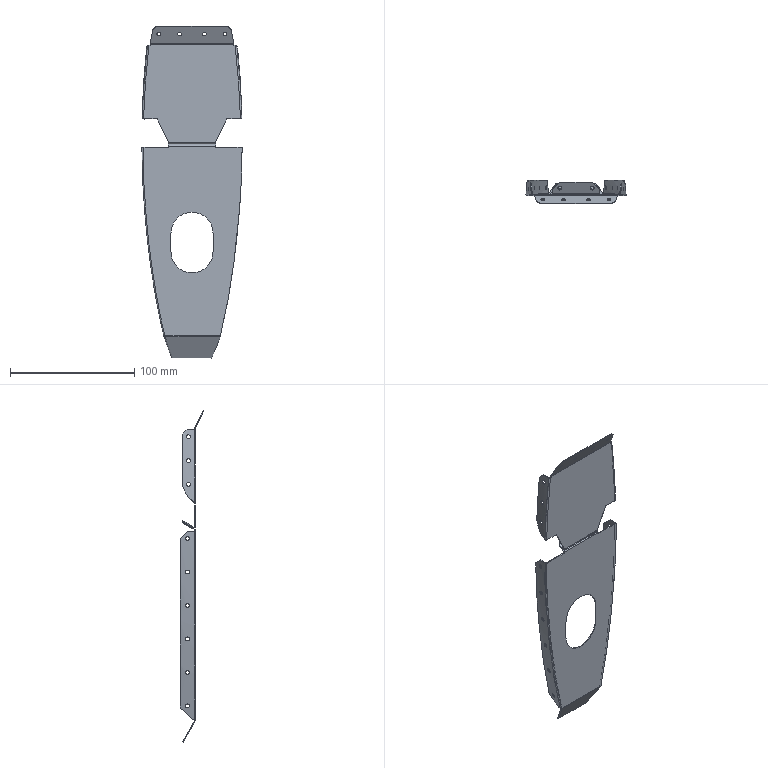Part | SolidWorks | features BaseBody 4 | 4 solids | 156 faces | box 80.774 x 19.265 x 267.636 mm | volume 10892 mm3 | plane 66 | cylinder 65 | spline 25 | commonest cylinder face diameters 3.2 x52 2 x8 34 x3 1 x2